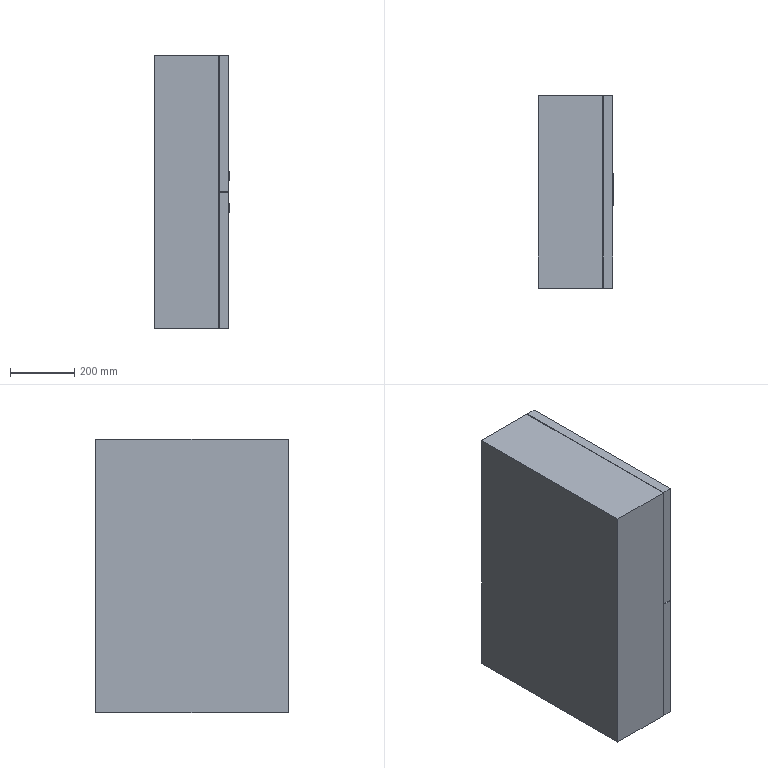Part | STEP file | Control Box | 7 solids | 54 faces | box 235 x 600 x 850 mm | volume 117277509 mm3 | plane 50 | cylinder 4 | commonest cylinder face diameters 14 x4